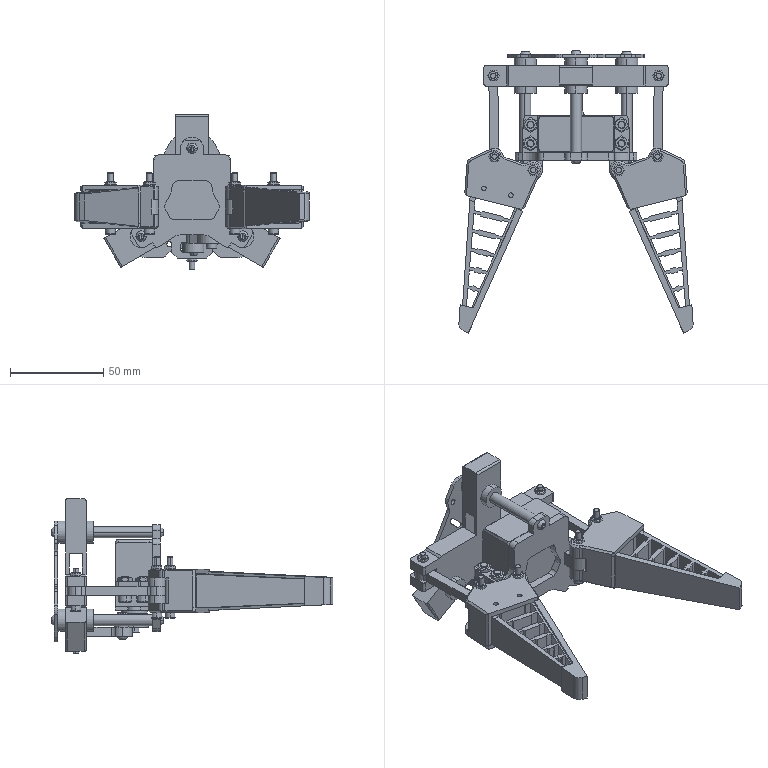Part | SolidWorks | 46 solids | 1733 faces | box 125.947 x 151.548 x 83 mm | volume 142512 mm3 | plane 957 | cylinder 478 | cone 222 | torus 44 | spline 18 | sphere 14 | commonest cylinder face diameters 3 x130 6 x64 0.1 x51 10 x25 2.5 x24 4 x22